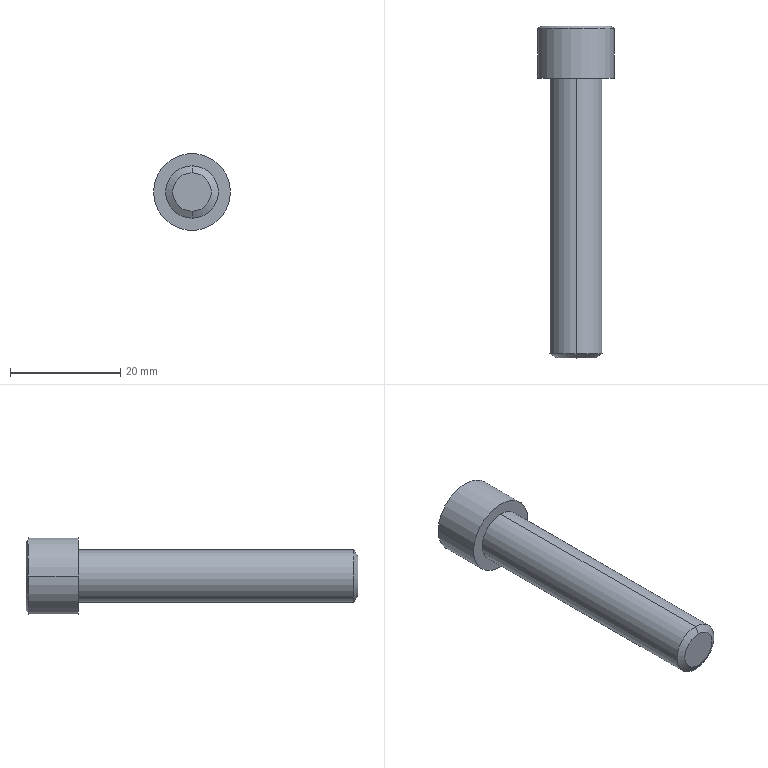Part | NX | features BREP 1 | 1 solid | 11 faces | box 13.97 x 60.325 x 13.97 mm | volume 5060 mm3 | cone 4 | cylinder 4 | plane 3 | commonest cylinder face diameters 9.525 x2 13.97 x2
STEP:
#1=CARTESIAN_POINT('',(0.,-50.8,3.493));
#2=VERTEX_POINT('',#1);
#3=CARTESIAN_POINT('',(0.,-50.8,-3.493));
#4=VERTEX_POINT('',#3);
#5=CARTESIAN_POINT('',(0.,-50.8,0.));
#6=DIRECTION('',(0.,-1.,0.));
#7=DIRECTION('',(0.,0.,1.));
#8=AXIS2_PLACEMENT_3D('',#5,#6,#7);
#9=CIRCLE('',#8,3.493);
#10=EDGE_CURVE('',#2,#4,#9,.T.);
#11=ORIENTED_EDGE('',*,*,#10,.T.);
#12=CARTESIAN_POINT('',(0.,-50.8,0.));
#13=DIRECTION('',(0.,-1.,0.));
#14=DIRECTION('',(0.,0.,-1.));
#15=AXIS2_PLACEMENT_3D('',#12,#13,#14);
#16=CIRCLE('',#15,3.493);
#17=EDGE_CURVE('',#4,#2,#16,.T.);
#18=ORIENTED_EDGE('',*,*,#17,.T.);
#19=EDGE_LOOP('',(#11,#18));
#20=FACE_BOUND('',#19,.T.);
#21=CARTESIAN_POINT('',(0.,-50.8,0.));
#22=DIRECTION('',(0.,-1.,0.));
#23=DIRECTION('',(0.,0.,-1.));
#24=AXIS2_PLACEMENT_3D('',#21,#22,#23);
#25=PLANE('',#24);
#26=ADVANCED_FACE('',(#20),#25,.T.);
#27=CARTESIAN_POINT('',(0.,-50.067,-4.763));
#28=VERTEX_POINT('',#27);
#29=CARTESIAN_POINT('',(0.,-50.8,-3.493));
#30=DIRECTION('',(0.,0.5,-0.866));
#31=VECTOR('',#30,1000.);
#32=LINE('',#29,#31);
#33=EDGE_CURVE('',#4,#28,#32,.T.);
#34=ORIENTED_EDGE('',*,*,#33,.T.);
#35=CARTESIAN_POINT('',(0.,-50.067,4.763));
#36=VERTEX_POINT('',#35);
#37=CARTESIAN_POINT('',(0.,-50.067,0.));
#38=DIRECTION('',(0.,-1.,0.));
#39=DIRECTION('',(0.,0.,-1.));
#40=AXIS2_PLACEMENT_3D('',#37,#38,#39);
#41=CIRCLE('',#40,4.763);
#42=EDGE_CURVE('',#28,#36,#41,.T.);
#43=ORIENTED_EDGE('',*,*,#42,.T.);
#44=CARTESIAN_POINT('',(0.,-50.8,3.493));
#45=DIRECTION('',(0.,0.5,0.866));
#46=VECTOR('',#45,1000.);
#47=LINE('',#44,#46);
#48=EDGE_CURVE('',#2,#36,#47,.T.);
#49=ORIENTED_EDGE('',*,*,#48,.F.);
#50=ORIENTED_EDGE('',*,*,#17,.F.);
#51=EDGE_LOOP('',(#34,#43,#49,#50));
#52=FACE_BOUND('',#51,.T.);
#53=CARTESIAN_POINT('',(0.,-50.433,0.));
#54=DIRECTION('',(0.,1.,0.));
#55=DIRECTION('',(0.,0.,1.));
#56=AXIS2_PLACEMENT_3D('',#53,#54,#55);
#57=CONICAL_SURFACE('',#56,4.128,1.047);
#58=ADVANCED_FACE('',(#52),#57,.T.);
#59=ORIENTED_EDGE('',*,*,#48,.T.);
#60=CARTESIAN_POINT('',(0.,-50.067,0.));
#61=DIRECTION('',(0.,-1.,0.));
#62=DIRECTION('',(0.,0.,1.));
#63=AXIS2_PLACEMENT_3D('',#60,#61,#62);
#64=CIRCLE('',#63,4.763);
#65=EDGE_CURVE('',#36,#28,#64,.T.);
#66=ORIENTED_EDGE('',*,*,#65,.T.);
#67=ORIENTED_EDGE('',*,*,#33,.F.);
#68=ORIENTED_EDGE('',*,*,#10,.F.);
#69=EDGE_LOOP('',(#59,#66,#67,#68));
#70=FACE_BOUND('',#69,.T.);
#71=CARTESIAN_POINT('',(0.,-50.433,0.));
#72=DIRECTION('',(0.,1.,0.));
#73=DIRECTION('',(0.,0.,1.));
#74=AXIS2_PLACEMENT_3D('',#71,#72,#73);
#75=CONICAL_SURFACE('',#74,4.128,1.047);
#76=ADVANCED_FACE('',(#70),#75,.T.);
#77=CARTESIAN_POINT('',(0.,0.,-4.763));
#78=VERTEX_POINT('',#77);
#79=CARTESIAN_POINT('',(0.,0.,-4.763));
#80=DIRECTION('',(0.,-1.,0.));
#81=VECTOR('',#80,1000.);
#82=LINE('',#79,#81);
#83=EDGE_CURVE('',#78,#28,#82,.T.);
#84=ORIENTED_EDGE('',*,*,#83,.T.);
#85=ORIENTED_EDGE('',*,*,#65,.F.);
#86=CARTESIAN_POINT('',(0.,0.,4.763));
#87=VERTEX_POINT('',#86);
#88=CARTESIAN_POINT('',(0.,0.,4.763));
#89=DIRECTION('',(0.,-1.,0.));
#90=VECTOR('',#89,1000.);
#91=LINE('',#88,#90);
#92=EDGE_CURVE('',#87,#36,#91,.T.);
#93=ORIENTED_EDGE('',*,*,#92,.F.);
#94=CARTESIAN_POINT('',(0.,0.,0.));
#95=DIRECTION('',(0.,-1.,0.));
#96=DIRECTION('',(0.,0.,1.));
#97=AXIS2_PLACEMENT_3D('',#94,#95,#96);
#98=CIRCLE('',#97,4.763);
#99=EDGE_CURVE('',#87,#78,#98,.T.);
#100=ORIENTED_EDGE('',*,*,#99,.T.);
#101=EDGE_LOOP('',(#84,#85,#93,#100));
#102=FACE_BOUND('',#101,.T.);
#103=CARTESIAN_POINT('',(0.,0.,0.));
#104=DIRECTION('',(0.,-1.,0.));
#105=DIRECTION('',(0.,0.,-1.));
#106=AXIS2_PLACEMENT_3D('',#103,#104,#105);
#107=CYLINDRICAL_SURFACE('',#106,4.763);
#108=ADVANCED_FACE('',(#102),#107,.T.);
#109=CARTESIAN_POINT('',(-6.985,0.,0.));
#110=VERTEX_POINT('',#109);
#111=CARTESIAN_POINT('',(6.985,0.,0.));
#112=VERTEX_POINT('',#111);
#113=CARTESIAN_POINT('',(0.,0.,0.));
#114=DIRECTION('',(0.,1.,0.));
#115=DIRECTION('',(-1.,0.,0.));
#116=AXIS2_PLACEMENT_3D('',#113,#114,#115);
#117=CIRCLE('',#116,6.985);
#118=EDGE_CURVE('',#110,#112,#117,.T.);
#119=ORIENTED_EDGE('',*,*,#118,.F.);
#120=CARTESIAN_POINT('',(0.,0.,0.));
#121=DIRECTION('',(0.,1.,0.));
#122=DIRECTION('',(1.,0.,0.));
#123=AXIS2_PLACEMENT_3D('',#120,#121,#122);
#124=CIRCLE('',#123,6.985);
#125=EDGE_CURVE('',#112,#110,#124,.T.);
#126=ORIENTED_EDGE('',*,*,#125,.F.);
#127=EDGE_LOOP('',(#119,#126));
#128=FACE_BOUND('',#127,.T.);
#129=ORIENTED_EDGE('',*,*,#99,.F.);
#130=CARTESIAN_POINT('',(0.,0.,0.));
#131=DIRECTION('',(0.,-1.,0.));
#132=DIRECTION('',(0.,0.,-1.));
#133=AXIS2_PLACEMENT_3D('',#130,#131,#132);
#134=CIRCLE('',#133,4.763);
#135=EDGE_CURVE('',#78,#87,#134,.T.);
#136=ORIENTED_EDGE('',*,*,#135,.F.);
#137=EDGE_LOOP('',(#129,#136));
#138=FACE_BOUND('',#137,.T.);
#139=CARTESIAN_POINT('',(0.,0.,0.));
#140=DIRECTION('',(0.,1.,0.));
#141=DIRECTION('',(1.,0.,0.));
#142=AXIS2_PLACEMENT_3D('',#139,#140,#141);
#143=PLANE('',#142);
#144=ADVANCED_FACE('',(#128,#138),#143,.F.);
#145=CARTESIAN_POINT('',(-6.985,9.085,0.));
#146=VERTEX_POINT('',#145);
#147=CARTESIAN_POINT('',(-6.985,0.,0.));
#148=DIRECTION('',(0.,1.,0.));
#149=VECTOR('',#148,1000.);
#150=LINE('',#147,#149);
#151=EDGE_CURVE('',#110,#146,#150,.T.);
#152=ORIENTED_EDGE('',*,*,#151,.T.);
#153=CARTESIAN_POINT('',(6.985,9.085,0.));
#154=VERTEX_POINT('',#153);
#155=CARTESIAN_POINT('',(0.,9.085,0.));
#156=DIRECTION('',(0.,1.,0.));
#157=DIRECTION('',(1.,0.,0.));
#158=AXIS2_PLACEMENT_3D('',#155,#156,#157);
#159=CIRCLE('',#158,6.985);
#160=EDGE_CURVE('',#154,#146,#159,.T.);
#161=ORIENTED_EDGE('',*,*,#160,.F.);
#162=CARTESIAN_POINT('',(6.985,0.,0.));
#163=DIRECTION('',(0.,1.,0.));
#164=VECTOR('',#163,1000.);
#165=LINE('',#162,#164);
#166=EDGE_CURVE('',#112,#154,#165,.T.);
#167=ORIENTED_EDGE('',*,*,#166,.F.);
#168=ORIENTED_EDGE('',*,*,#125,.T.);
#169=EDGE_LOOP('',(#152,#161,#167,#168));
#170=FACE_BOUND('',#169,.T.);
#171=CARTESIAN_POINT('',(0.,0.,0.));
#172=DIRECTION('',(0.,1.,0.));
#173=DIRECTION('',(1.,0.,0.));
#174=AXIS2_PLACEMENT_3D('',#171,#172,#173);
#175=CYLINDRICAL_SURFACE('',#174,6.985);
#176=ADVANCED_FACE('',(#170),#175,.T.);
#177=ORIENTED_EDGE('',*,*,#166,.T.);
#178=CARTESIAN_POINT('',(0.,9.085,0.));
#179=DIRECTION('',(0.,1.,0.));
#180=DIRECTION('',(-1.,0.,0.));
#181=AXIS2_PLACEMENT_3D('',#178,#179,#180);
#182=CIRCLE('',#181,6.985);
#183=EDGE_CURVE('',#146,#154,#182,.T.);
#184=ORIENTED_EDGE('',*,*,#183,.F.);
#185=ORIENTED_EDGE('',*,*,#151,.F.);
#186=ORIENTED_EDGE('',*,*,#118,.T.);
#187=EDGE_LOOP('',(#177,#184,#185,#186));
#188=FACE_BOUND('',#187,.T.);
#189=CARTESIAN_POINT('',(0.,0.,0.));
#190=DIRECTION('',(0.,1.,0.));
#191=DIRECTION('',(1.,0.,0.));
#192=AXIS2_PLACEMENT_3D('',#189,#190,#191);
#193=CYLINDRICAL_SURFACE('',#192,6.985);
#194=ADVANCED_FACE('',(#188),#193,.T.);
#195=CARTESIAN_POINT('',(-6.223,9.525,0.));
#196=VERTEX_POINT('',#195);
#197=CARTESIAN_POINT('',(-6.223,9.525,0.));
#198=DIRECTION('',(-0.866,-0.5,0.));
#199=VECTOR('',#198,1000.);
#200=LINE('',#197,#199);
#201=EDGE_CURVE('',#196,#146,#200,.T.);
#202=ORIENTED_EDGE('',*,*,#201,.T.);
#203=ORIENTED_EDGE('',*,*,#183,.T.);
#204=CARTESIAN_POINT('',(6.223,9.525,0.));
#205=VERTEX_POINT('',#204);
#206=CARTESIAN_POINT('',(6.223,9.525,0.));
#207=DIRECTION('',(0.866,-0.5,0.));
#208=VECTOR('',#207,1000.);
#209=LINE('',#206,#208);
#210=EDGE_CURVE('',#205,#154,#209,.T.);
#211=ORIENTED_EDGE('',*,*,#210,.F.);
#212=CARTESIAN_POINT('',(0.,9.525,0.));
#213=DIRECTION('',(0.,1.,0.));
#214=DIRECTION('',(-1.,0.,0.));
#215=AXIS2_PLACEMENT_3D('',#212,#213,#214);
#216=CIRCLE('',#215,6.223);
#217=EDGE_CURVE('',#196,#205,#216,.T.);
#218=ORIENTED_EDGE('',*,*,#217,.F.);
#219=EDGE_LOOP('',(#202,#203,#211,#218));
#220=FACE_BOUND('',#219,.T.);
#221=CARTESIAN_POINT('',(0.,9.305,0.));
#222=DIRECTION('',(0.,-1.,0.));
#223=DIRECTION('',(-1.,0.,0.));
#224=AXIS2_PLACEMENT_3D('',#221,#222,#223);
#225=CONICAL_SURFACE('',#224,6.604,1.047);
#226=ADVANCED_FACE('',(#220),#225,.T.);
#227=ORIENTED_EDGE('',*,*,#217,.T.);
#228=CARTESIAN_POINT('',(0.,9.525,0.));
#229=DIRECTION('',(0.,1.,0.));
#230=DIRECTION('',(1.,0.,0.));
#231=AXIS2_PLACEMENT_3D('',#228,#229,#230);
#232=CIRCLE('',#231,6.223);
#233=EDGE_CURVE('',#205,#196,#232,.T.);
#234=ORIENTED_EDGE('',*,*,#233,.T.);
#235=EDGE_LOOP('',(#227,#234));
#236=FACE_BOUND('',#235,.T.);
#237=CARTESIAN_POINT('',(0.,9.525,0.));
#238=DIRECTION('',(0.,1.,0.));
#239=DIRECTION('',(1.,0.,0.));
#240=AXIS2_PLACEMENT_3D('',#237,#238,#239);
#241=PLANE('',#240);
#242=ADVANCED_FACE('',(#236),#241,.T.);
#243=ORIENTED_EDGE('',*,*,#210,.T.);
#244=ORIENTED_EDGE('',*,*,#160,.T.);
#245=ORIENTED_EDGE('',*,*,#201,.F.);
#246=ORIENTED_EDGE('',*,*,#233,.F.);
#247=EDGE_LOOP('',(#243,#244,#245,#246));
#248=FACE_BOUND('',#247,.T.);
#249=CARTESIAN_POINT('',(0.,9.305,0.));
#250=DIRECTION('',(0.,-1.,0.));
#251=DIRECTION('',(-1.,0.,0.));
#252=AXIS2_PLACEMENT_3D('',#249,#250,#251);
#253=CONICAL_SURFACE('',#252,6.604,1.047);
#254=ADVANCED_FACE('',(#248),#253,.T.);
#255=ORIENTED_EDGE('',*,*,#92,.T.);
#256=ORIENTED_EDGE('',*,*,#42,.F.);
#257=ORIENTED_EDGE('',*,*,#83,.F.);
#258=ORIENTED_EDGE('',*,*,#135,.T.);
#259=EDGE_LOOP('',(#255,#256,#257,#258));
#260=FACE_BOUND('',#259,.T.);
#261=CARTESIAN_POINT('',(0.,0.,0.));
#262=DIRECTION('',(0.,-1.,0.));
#263=DIRECTION('',(0.,0.,-1.));
#264=AXIS2_PLACEMENT_3D('',#261,#262,#263);
#265=CYLINDRICAL_SURFACE('',#264,4.763);
#266=ADVANCED_FACE('',(#260),#265,.T.);
#267=CLOSED_SHELL('',(#26,#58,#76,#108,#144,#176,#194,#226,#242,#254,#266));
#268=MANIFOLD_SOLID_BREP('',#267);
#269=(LENGTH_UNIT()NAMED_UNIT(*)SI_UNIT(.MILLI.,.METRE.));
#270=UNCERTAINTY_MEASURE_WITH_UNIT(LENGTH_MEASURE(0.00001),#269,'','');
#271=(NAMED_UNIT(*)PLANE_ANGLE_UNIT()SI_UNIT($,.RADIAN.));
#272=(NAMED_UNIT(*)SI_UNIT($,.STERADIAN.)SOLID_ANGLE_UNIT());
#273=(GEOMETRIC_REPRESENTATION_CONTEXT(3)GLOBAL_UNCERTAINTY_ASSIGNED_CONTEXT((#270))GLOBAL_UNIT_ASSIGNED_CONTEXT((#269,#271,#272))REPRESENTATION_CONTEXT('',''));
#274=ADVANCED_BREP_SHAPE_REPRESENTATION('',(#268),#273);